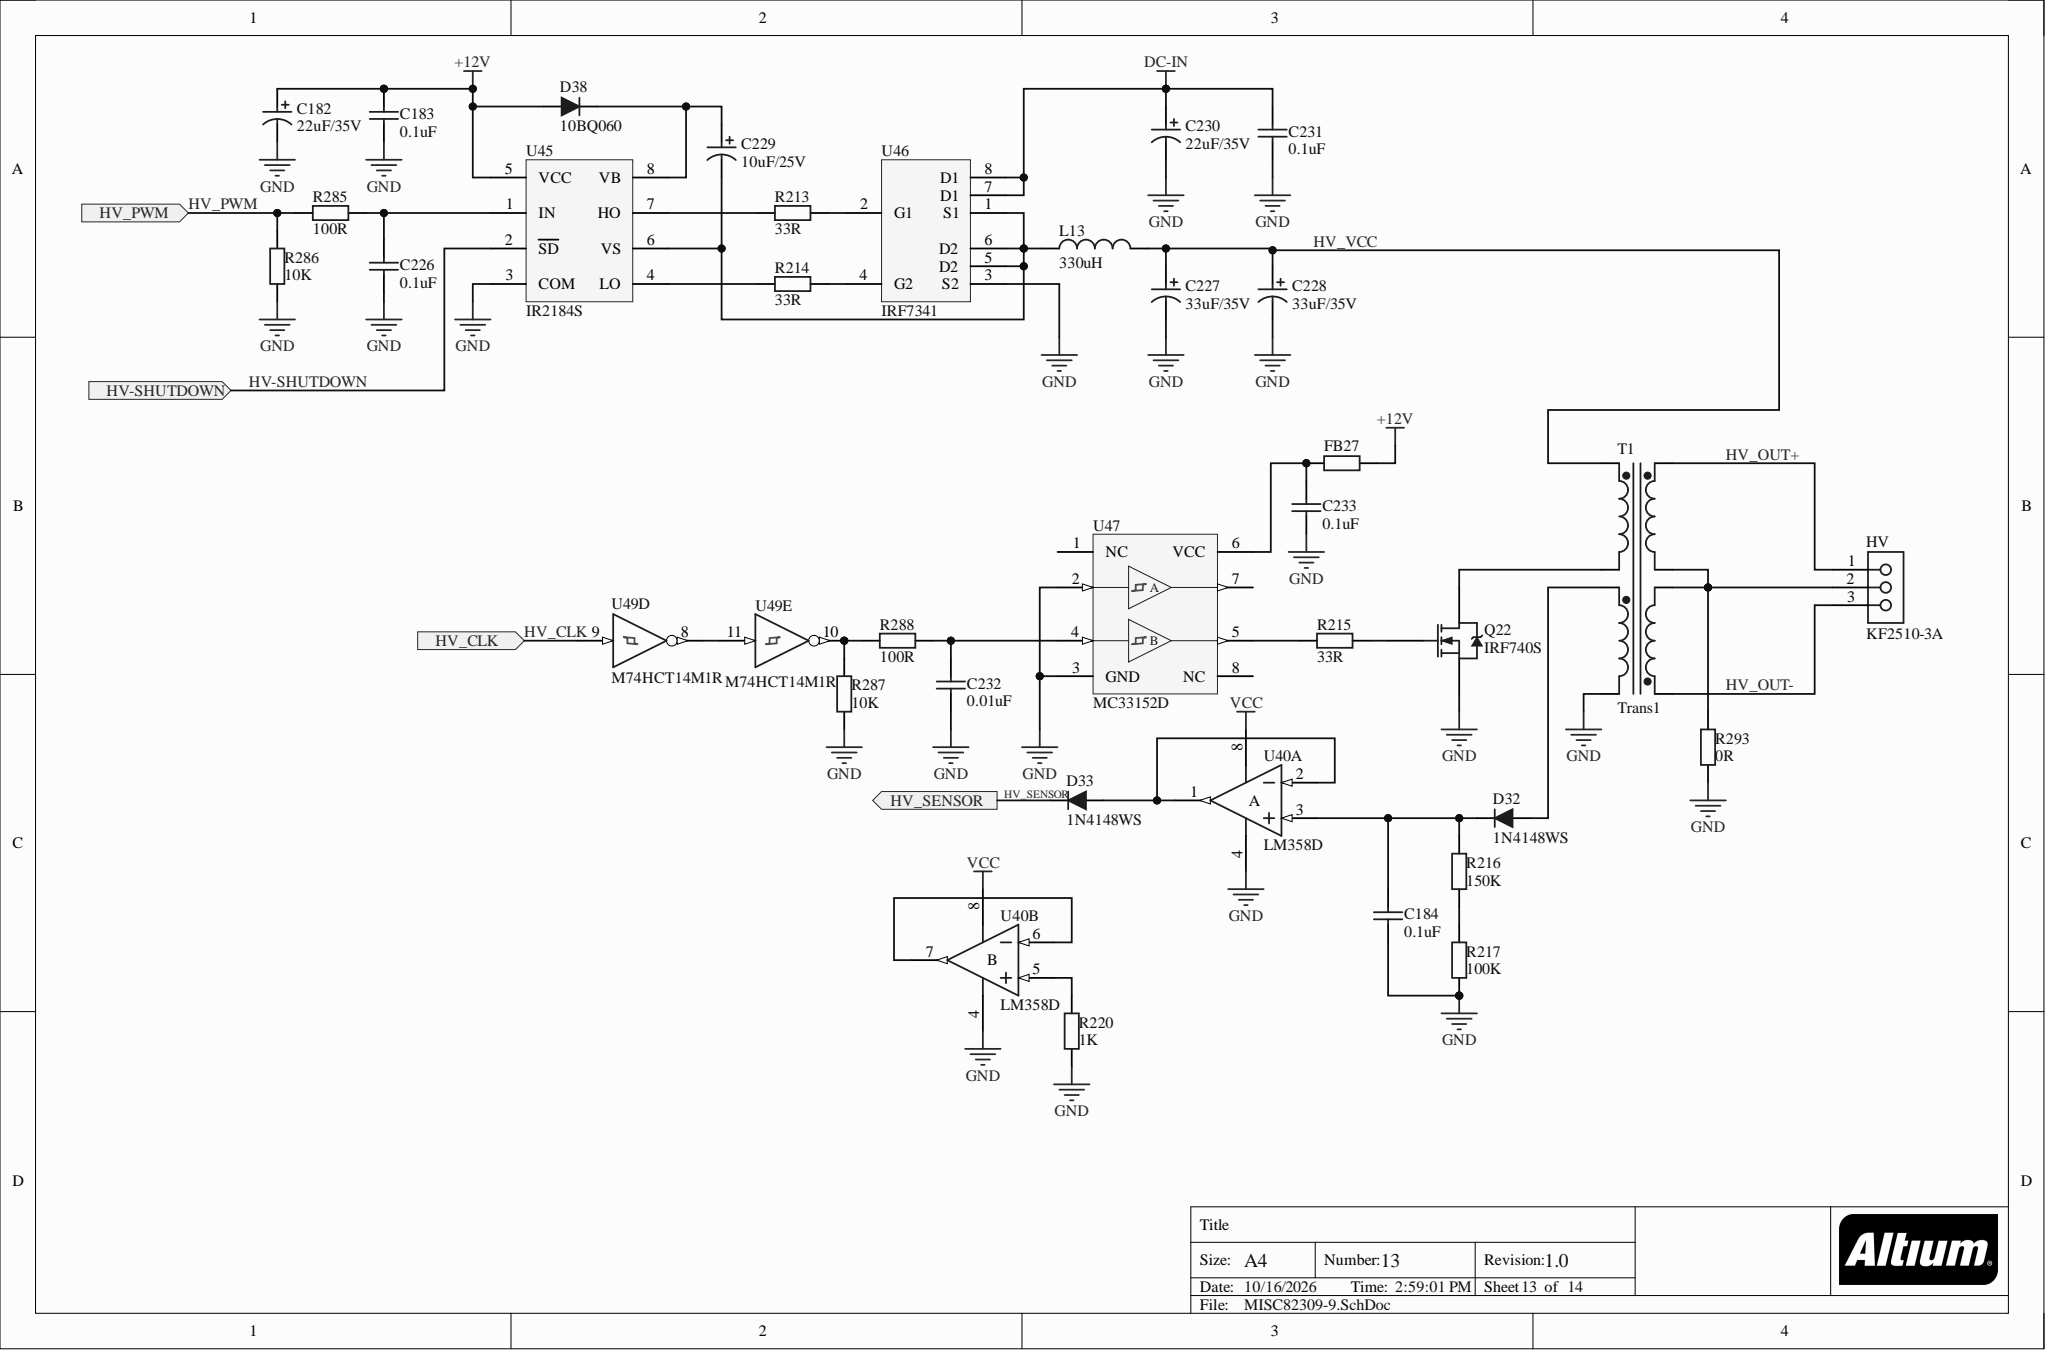Circuit board | Altium Designer | 747 parts | 576 nets | one sheet of the schematic
Parts on this sheet (reference | value | footprint):
C182 | 22uF/35V | CAP-ALU-6_3X5_4
C183 | 0.1uF | CAP_0805
C184 | 0.1uF | CAP_0805
C226 | 0.1uF | CAP_0603
C227 | 33uF/35V | CAP-ALU-6_3X5_4
C228 | 33uF/35V | CAP-ALU-6_3X5_4
C229 | 10uF/25V | CAP-ALU-5X5_4
C230 | 22uF/35V | CAP-ALU-6_3X5_4
C231 | 0.1uF | CAP_0805
C232 | 0.01uF | CAP_0603
C233 | 0.1uF | CAP_0805
D32 | 1N4148WS | SOD323
D33 | 1N4148WS | SOD323
D38 | 10BQ060 | DO-214AA-L
HV | KF2510-3A | KF2510-3A
L13 | 330uH | PBS5022
Q22 | IRF740S | D2PAK_N
R213 | 33R | RES_0603
R214 | 33R | RES_0603
R215 | 33R | RES_0805
R216 | 150K | R0805
R217 | 100K | R0805
R220 | 1K | R0805
R285 | 100R | RES_0603
R286 | 10K | RES_0603
R287 | 10K | RES_0603
R288 | 100R | RES_0603
R293 | 0R | RES_0805
T1 | Trans1 | RM8
U45 | IR2184S | SOIC_8N
U46 | IRF7341 | SOIC_8N
U47 | MC33152D | 751-05_N
Nets of these parts (net: part-pin ...):
NetR287_2: R287-2 R288-1
NetR220_1: R220-1
NetR216_1: R216-1 R217-1
NetR215_2: R215-2 U47-5
NetR214_2: R214-2 U45-4
NetR214_1: R214-1 U46-4
NetR213_2: R213-2 U45-7
NetR213_1: R213-1 U46-2
NetQ22_2: Q22-2 T1-1
NetQ22_1: Q22-1 R215-1
NetHV_2: HV-2 R293-1 T1-11 T1-12
NetD33_1: D33-1
NetD32_1: D32-1 T1-4
NetC233_2: C233-2 U47-6
NetC232_2: C232-2 R288-2 U47-4
NetC229_2: C229-2 D38-2 U45-8
NetC229_1: C229-1 L13-1 U45-6 U46-1 U46-5 U46-6
NetC226_2: C226-2 R285-2 U45-1
NetC184_2: C184-2 D32-2 R216-2
HV_VCC: C227-2 C228-2 L13-2 T1-2
HV_SENSOR: D33-2
HV_PWM: R285-1 R286-2
HV_OUT-: HV-3 T1-8
HV_OUT+: HV-1 T1-7
HV-SHUTDOWN: U45-2
GND: C182-1 C183-1 C184-1 C226-1 C227-1 C228-1 C230-1 C231-1 C232-1 C233-1 Q22-3 R217-2 R220-2 R286-1 R287-1 R293-2 T1-3 U45-3 U46-3 U47-2 U47-3
DC-IN: C230-2 C231-2 U46-7 U46-8
+12V: C182-2 C183-2 D38-1 U45-5